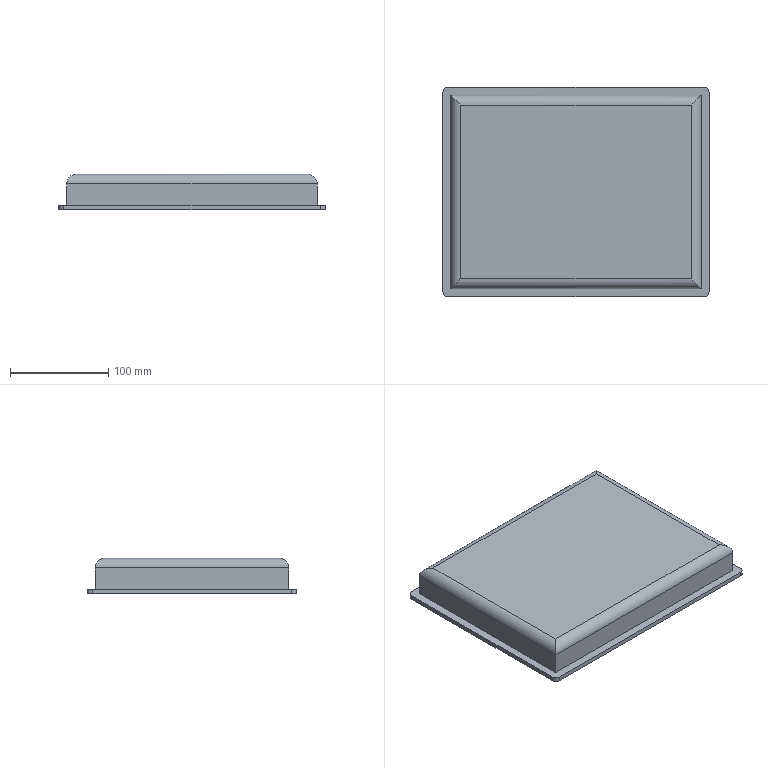Part | SolidWorks | features Fillet 2, ICE 2, Extrusion 1 | 1 solid | 24 faces | box 271 x 213 x 36.36 mm | volume 1748728 mm3 | plane 16 | cylinder 8 | commonest cylinder face diameters 10 x4 20 x4
STEP:
#1=CARTESIAN_POINT('',(0.,-5.,4.5));
#2=VERTEX_POINT('',#1);
#3=CARTESIAN_POINT('',(0.,-208.,4.5));
#4=VERTEX_POINT('',#3);
#5=CARTESIAN_POINT('',(0.,0.,4.5));
#6=DIRECTION('',(0.,-1.,0.));
#7=VECTOR('',#6,1000.);
#8=LINE('',#5,#7);
#9=EDGE_CURVE('',#2,#4,#8,.T.);
#10=ORIENTED_EDGE('',*,*,#9,.T.);
#11=CARTESIAN_POINT('',(5.,-213.,4.5));
#12=VERTEX_POINT('',#11);
#13=CARTESIAN_POINT('',(5.,-208.,4.5));
#14=DIRECTION('',(0.,0.,1.));
#15=DIRECTION('',(1.,0.,0.));
#16=AXIS2_PLACEMENT_3D('',#13,#14,#15);
#17=CIRCLE('',#16,5.);
#18=EDGE_CURVE('',#4,#12,#17,.T.);
#19=ORIENTED_EDGE('',*,*,#18,.T.);
#20=CARTESIAN_POINT('',(266.,-213.,4.5));
#21=VERTEX_POINT('',#20);
#22=CARTESIAN_POINT('',(0.,-213.,4.5));
#23=DIRECTION('',(1.,0.,0.));
#24=VECTOR('',#23,1000.);
#25=LINE('',#22,#24);
#26=EDGE_CURVE('',#12,#21,#25,.T.);
#27=ORIENTED_EDGE('',*,*,#26,.T.);
#28=CARTESIAN_POINT('',(271.,-208.,4.5));
#29=VERTEX_POINT('',#28);
#30=CARTESIAN_POINT('',(266.,-208.,4.5));
#31=DIRECTION('',(0.,0.,1.));
#32=DIRECTION('',(1.,0.,0.));
#33=AXIS2_PLACEMENT_3D('',#30,#31,#32);
#34=CIRCLE('',#33,5.);
#35=EDGE_CURVE('',#21,#29,#34,.T.);
#36=ORIENTED_EDGE('',*,*,#35,.T.);
#37=CARTESIAN_POINT('',(271.,-5.,4.5));
#38=VERTEX_POINT('',#37);
#39=CARTESIAN_POINT('',(271.,0.,4.5));
#40=DIRECTION('',(0.,1.,0.));
#41=VECTOR('',#40,1000.);
#42=LINE('',#39,#41);
#43=EDGE_CURVE('',#29,#38,#42,.T.);
#44=ORIENTED_EDGE('',*,*,#43,.T.);
#45=CARTESIAN_POINT('',(266.,0.,4.5));
#46=VERTEX_POINT('',#45);
#47=CARTESIAN_POINT('',(266.,-5.,4.5));
#48=DIRECTION('',(0.,0.,1.));
#49=DIRECTION('',(1.,0.,0.));
#50=AXIS2_PLACEMENT_3D('',#47,#48,#49);
#51=CIRCLE('',#50,5.);
#52=EDGE_CURVE('',#38,#46,#51,.T.);
#53=ORIENTED_EDGE('',*,*,#52,.T.);
#54=CARTESIAN_POINT('',(5.,0.,4.5));
#55=VERTEX_POINT('',#54);
#56=CARTESIAN_POINT('',(0.,0.,4.5));
#57=DIRECTION('',(-1.,0.,0.));
#58=VECTOR('',#57,1000.);
#59=LINE('',#56,#58);
#60=EDGE_CURVE('',#46,#55,#59,.T.);
#61=ORIENTED_EDGE('',*,*,#60,.T.);
#62=CARTESIAN_POINT('',(5.,-5.,4.5));
#63=DIRECTION('',(0.,0.,1.));
#64=DIRECTION('',(1.,0.,0.));
#65=AXIS2_PLACEMENT_3D('',#62,#63,#64);
#66=CIRCLE('',#65,5.);
#67=EDGE_CURVE('',#55,#2,#66,.T.);
#68=ORIENTED_EDGE('',*,*,#67,.T.);
#69=EDGE_LOOP('',(#10,#19,#27,#36,#44,#53,#61,#68));
#70=FACE_OUTER_BOUND('',#69,.T.);
#71=CARTESIAN_POINT('',(263.,-8.,4.5));
#72=VERTEX_POINT('',#71);
#73=CARTESIAN_POINT('',(8.,-8.,4.5));
#74=VERTEX_POINT('',#73);
#75=CARTESIAN_POINT('',(8.,-8.,4.5));
#76=DIRECTION('',(-1.,0.,0.));
#77=VECTOR('',#76,1000.);
#78=LINE('',#75,#77);
#79=EDGE_CURVE('',#72,#74,#78,.T.);
#80=ORIENTED_EDGE('',*,*,#79,.F.);
#81=CARTESIAN_POINT('',(263.,-205.,4.5));
#82=VERTEX_POINT('',#81);
#83=CARTESIAN_POINT('',(263.,-8.,4.5));
#84=DIRECTION('',(0.,1.,0.));
#85=VECTOR('',#84,1000.);
#86=LINE('',#83,#85);
#87=EDGE_CURVE('',#82,#72,#86,.T.);
#88=ORIENTED_EDGE('',*,*,#87,.F.);
#89=CARTESIAN_POINT('',(8.,-205.,4.5));
#90=VERTEX_POINT('',#89);
#91=CARTESIAN_POINT('',(8.,-205.,4.5));
#92=DIRECTION('',(1.,0.,0.));
#93=VECTOR('',#92,1000.);
#94=LINE('',#91,#93);
#95=EDGE_CURVE('',#90,#82,#94,.T.);
#96=ORIENTED_EDGE('',*,*,#95,.F.);
#97=CARTESIAN_POINT('',(8.,-8.,4.5));
#98=DIRECTION('',(0.,-1.,0.));
#99=VECTOR('',#98,1000.);
#100=LINE('',#97,#99);
#101=EDGE_CURVE('',#74,#90,#100,.T.);
#102=ORIENTED_EDGE('',*,*,#101,.F.);
#103=EDGE_LOOP('',(#80,#88,#96,#102));
#104=FACE_BOUND('',#103,.T.);
#105=CARTESIAN_POINT('',(0.,0.,4.5));
#106=DIRECTION('',(0.,0.,1.));
#107=DIRECTION('',(1.,0.,0.));
#108=AXIS2_PLACEMENT_3D('',#105,#106,#107);
#109=PLANE('',#108);
#110=ADVANCED_FACE('',(#70,#104),#109,.T.);
#111=CARTESIAN_POINT('',(0.,-5.,0.));
#112=VERTEX_POINT('',#111);
#113=CARTESIAN_POINT('',(0.,-208.,0.));
#114=VERTEX_POINT('',#113);
#115=CARTESIAN_POINT('',(0.,0.,0.));
#116=DIRECTION('',(0.,-1.,0.));
#117=VECTOR('',#116,1000.);
#118=LINE('',#115,#117);
#119=EDGE_CURVE('',#112,#114,#118,.T.);
#120=ORIENTED_EDGE('',*,*,#119,.T.);
#121=CARTESIAN_POINT('',(0.,-208.,4.5));
#122=DIRECTION('',(0.,0.,1.));
#123=VECTOR('',#122,1000.);
#124=LINE('',#121,#123);
#125=EDGE_CURVE('',#114,#4,#124,.T.);
#126=ORIENTED_EDGE('',*,*,#125,.T.);
#127=ORIENTED_EDGE('',*,*,#9,.F.);
#128=CARTESIAN_POINT('',(0.,-5.,4.5));
#129=DIRECTION('',(0.,0.,-1.));
#130=VECTOR('',#129,1000.);
#131=LINE('',#128,#130);
#132=EDGE_CURVE('',#2,#112,#131,.T.);
#133=ORIENTED_EDGE('',*,*,#132,.T.);
#134=EDGE_LOOP('',(#120,#126,#127,#133));
#135=FACE_OUTER_BOUND('',#134,.T.);
#136=CARTESIAN_POINT('',(0.,0.,4.5));
#137=DIRECTION('',(1.,0.,0.));
#138=DIRECTION('',(0.,1.,0.));
#139=AXIS2_PLACEMENT_3D('',#136,#137,#138);
#140=PLANE('',#139);
#141=ADVANCED_FACE('',(#135),#140,.F.);
#142=ORIENTED_EDGE('',*,*,#26,.F.);
#143=CARTESIAN_POINT('',(5.,-213.,0.));
#144=VERTEX_POINT('',#143);
#145=CARTESIAN_POINT('',(5.,-213.,4.5));
#146=DIRECTION('',(0.,0.,-1.));
#147=VECTOR('',#146,1000.);
#148=LINE('',#145,#147);
#149=EDGE_CURVE('',#12,#144,#148,.T.);
#150=ORIENTED_EDGE('',*,*,#149,.T.);
#151=CARTESIAN_POINT('',(266.,-213.,0.));
#152=VERTEX_POINT('',#151);
#153=CARTESIAN_POINT('',(0.,-213.,0.));
#154=DIRECTION('',(1.,0.,0.));
#155=VECTOR('',#154,1000.);
#156=LINE('',#153,#155);
#157=EDGE_CURVE('',#144,#152,#156,.T.);
#158=ORIENTED_EDGE('',*,*,#157,.T.);
#159=CARTESIAN_POINT('',(266.,-213.,4.5));
#160=DIRECTION('',(0.,0.,1.));
#161=VECTOR('',#160,1000.);
#162=LINE('',#159,#161);
#163=EDGE_CURVE('',#152,#21,#162,.T.);
#164=ORIENTED_EDGE('',*,*,#163,.T.);
#165=EDGE_LOOP('',(#142,#150,#158,#164));
#166=FACE_OUTER_BOUND('',#165,.T.);
#167=CARTESIAN_POINT('',(0.,-213.,4.5));
#168=DIRECTION('',(0.,1.,0.));
#169=DIRECTION('',(0.,0.,1.));
#170=AXIS2_PLACEMENT_3D('',#167,#168,#169);
#171=PLANE('',#170);
#172=ADVANCED_FACE('',(#166),#171,.F.);
#173=ORIENTED_EDGE('',*,*,#43,.F.);
#174=CARTESIAN_POINT('',(271.,-208.,0.));
#175=VERTEX_POINT('',#174);
#176=CARTESIAN_POINT('',(271.,-208.,4.5));
#177=DIRECTION('',(0.,0.,-1.));
#178=VECTOR('',#177,1000.);
#179=LINE('',#176,#178);
#180=EDGE_CURVE('',#29,#175,#179,.T.);
#181=ORIENTED_EDGE('',*,*,#180,.T.);
#182=CARTESIAN_POINT('',(271.,-5.,0.));
#183=VERTEX_POINT('',#182);
#184=CARTESIAN_POINT('',(271.,0.,0.));
#185=DIRECTION('',(0.,1.,0.));
#186=VECTOR('',#185,1000.);
#187=LINE('',#184,#186);
#188=EDGE_CURVE('',#175,#183,#187,.T.);
#189=ORIENTED_EDGE('',*,*,#188,.T.);
#190=CARTESIAN_POINT('',(271.,-5.,4.5));
#191=DIRECTION('',(0.,0.,1.));
#192=VECTOR('',#191,1000.);
#193=LINE('',#190,#192);
#194=EDGE_CURVE('',#183,#38,#193,.T.);
#195=ORIENTED_EDGE('',*,*,#194,.T.);
#196=EDGE_LOOP('',(#173,#181,#189,#195));
#197=FACE_OUTER_BOUND('',#196,.T.);
#198=CARTESIAN_POINT('',(271.,0.,4.5));
#199=DIRECTION('',(-1.,0.,0.));
#200=DIRECTION('',(0.,0.,1.));
#201=AXIS2_PLACEMENT_3D('',#198,#199,#200);
#202=PLANE('',#201);
#203=ADVANCED_FACE('',(#197),#202,.F.);
#204=ORIENTED_EDGE('',*,*,#60,.F.);
#205=CARTESIAN_POINT('',(266.,0.,0.));
#206=VERTEX_POINT('',#205);
#207=CARTESIAN_POINT('',(266.,0.,4.5));
#208=DIRECTION('',(0.,0.,-1.));
#209=VECTOR('',#208,1000.);
#210=LINE('',#207,#209);
#211=EDGE_CURVE('',#46,#206,#210,.T.);
#212=ORIENTED_EDGE('',*,*,#211,.T.);
#213=CARTESIAN_POINT('',(5.,0.,0.));
#214=VERTEX_POINT('',#213);
#215=CARTESIAN_POINT('',(0.,0.,0.));
#216=DIRECTION('',(-1.,0.,0.));
#217=VECTOR('',#216,1000.);
#218=LINE('',#215,#217);
#219=EDGE_CURVE('',#206,#214,#218,.T.);
#220=ORIENTED_EDGE('',*,*,#219,.T.);
#221=CARTESIAN_POINT('',(5.,0.,4.5));
#222=DIRECTION('',(0.,0.,1.));
#223=VECTOR('',#222,1000.);
#224=LINE('',#221,#223);
#225=EDGE_CURVE('',#214,#55,#224,.T.);
#226=ORIENTED_EDGE('',*,*,#225,.T.);
#227=EDGE_LOOP('',(#204,#212,#220,#226));
#228=FACE_OUTER_BOUND('',#227,.T.);
#229=CARTESIAN_POINT('',(0.,0.,4.5));
#230=DIRECTION('',(0.,-1.,0.));
#231=DIRECTION('',(0.,0.,-1.));
#232=AXIS2_PLACEMENT_3D('',#229,#230,#231);
#233=PLANE('',#232);
#234=ADVANCED_FACE('',(#228),#233,.F.);
#235=CARTESIAN_POINT('',(25.5,-36.5,0.));
#236=VERTEX_POINT('',#235);
#237=CARTESIAN_POINT('',(245.5,-36.5,0.));
#238=VERTEX_POINT('',#237);
#239=CARTESIAN_POINT('',(245.5,-36.5,0.));
#240=DIRECTION('',(1.,0.,0.));
#241=VECTOR('',#240,1000.);
#242=LINE('',#239,#241);
#243=EDGE_CURVE('',#236,#238,#242,.T.);
#244=ORIENTED_EDGE('',*,*,#243,.F.);
#245=CARTESIAN_POINT('',(25.5,-176.5,0.));
#246=VERTEX_POINT('',#245);
#247=CARTESIAN_POINT('',(25.5,-36.5,0.));
#248=DIRECTION('',(0.,1.,0.));
#249=VECTOR('',#248,1000.);
#250=LINE('',#247,#249);
#251=EDGE_CURVE('',#246,#236,#250,.T.);
#252=ORIENTED_EDGE('',*,*,#251,.F.);
#253=CARTESIAN_POINT('',(245.5,-176.5,0.));
#254=VERTEX_POINT('',#253);
#255=CARTESIAN_POINT('',(245.5,-176.5,0.));
#256=DIRECTION('',(-1.,0.,0.));
#257=VECTOR('',#256,1000.);
#258=LINE('',#255,#257);
#259=EDGE_CURVE('',#254,#246,#258,.T.);
#260=ORIENTED_EDGE('',*,*,#259,.F.);
#261=CARTESIAN_POINT('',(245.5,-36.5,0.));
#262=DIRECTION('',(0.,-1.,0.));
#263=VECTOR('',#262,1000.);
#264=LINE('',#261,#263);
#265=EDGE_CURVE('',#238,#254,#264,.T.);
#266=ORIENTED_EDGE('',*,*,#265,.F.);
#267=EDGE_LOOP('',(#244,#252,#260,#266));
#268=FACE_BOUND('',#267,.T.);
#269=ORIENTED_EDGE('',*,*,#157,.F.);
#270=CARTESIAN_POINT('',(5.,-208.,0.));
#271=DIRECTION('',(0.,0.,-1.));
#272=DIRECTION('',(1.,0.,0.));
#273=AXIS2_PLACEMENT_3D('',#270,#271,#272);
#274=CIRCLE('',#273,5.);
#275=EDGE_CURVE('',#144,#114,#274,.T.);
#276=ORIENTED_EDGE('',*,*,#275,.T.);
#277=ORIENTED_EDGE('',*,*,#119,.F.);
#278=CARTESIAN_POINT('',(5.,-5.,0.));
#279=DIRECTION('',(0.,0.,-1.));
#280=DIRECTION('',(1.,0.,0.));
#281=AXIS2_PLACEMENT_3D('',#278,#279,#280);
#282=CIRCLE('',#281,5.);
#283=EDGE_CURVE('',#112,#214,#282,.T.);
#284=ORIENTED_EDGE('',*,*,#283,.T.);
#285=ORIENTED_EDGE('',*,*,#219,.F.);
#286=CARTESIAN_POINT('',(266.,-5.,0.));
#287=DIRECTION('',(0.,0.,-1.));
#288=DIRECTION('',(1.,0.,0.));
#289=AXIS2_PLACEMENT_3D('',#286,#287,#288);
#290=CIRCLE('',#289,5.);
#291=EDGE_CURVE('',#206,#183,#290,.T.);
#292=ORIENTED_EDGE('',*,*,#291,.T.);
#293=ORIENTED_EDGE('',*,*,#188,.F.);
#294=CARTESIAN_POINT('',(266.,-208.,0.));
#295=DIRECTION('',(0.,0.,-1.));
#296=DIRECTION('',(1.,0.,0.));
#297=AXIS2_PLACEMENT_3D('',#294,#295,#296);
#298=CIRCLE('',#297,5.);
#299=EDGE_CURVE('',#175,#152,#298,.T.);
#300=ORIENTED_EDGE('',*,*,#299,.T.);
#301=EDGE_LOOP('',(#269,#276,#277,#284,#285,#292,#293,#300));
#302=FACE_OUTER_BOUND('',#301,.T.);
#303=CARTESIAN_POINT('',(0.,0.,0.));
#304=DIRECTION('',(0.,0.,1.));
#305=DIRECTION('',(1.,0.,0.));
#306=AXIS2_PLACEMENT_3D('',#303,#304,#305);
#307=PLANE('',#306);
#308=ADVANCED_FACE('',(#268,#302),#307,.F.);
#309=CARTESIAN_POINT('',(263.,-8.,26.36));
#310=VERTEX_POINT('',#309);
#311=CARTESIAN_POINT('',(263.,-8.,36.36));
#312=DIRECTION('',(0.,0.,-1.));
#313=VECTOR('',#312,1000.);
#314=LINE('',#311,#313);
#315=EDGE_CURVE('',#310,#72,#314,.T.);
#316=ORIENTED_EDGE('',*,*,#315,.F.);
#317=CARTESIAN_POINT('',(263.,-205.,26.36));
#318=VERTEX_POINT('',#317);
#319=CARTESIAN_POINT('',(263.,-205.,26.36));
#320=DIRECTION('',(0.,-1.,0.));
#321=VECTOR('',#320,1000.);
#322=LINE('',#319,#321);
#323=EDGE_CURVE('',#310,#318,#322,.T.);
#324=ORIENTED_EDGE('',*,*,#323,.T.);
#325=CARTESIAN_POINT('',(263.,-205.,36.36));
#326=DIRECTION('',(0.,0.,-1.));
#327=VECTOR('',#326,1000.);
#328=LINE('',#325,#327);
#329=EDGE_CURVE('',#318,#82,#328,.T.);
#330=ORIENTED_EDGE('',*,*,#329,.T.);
#331=ORIENTED_EDGE('',*,*,#87,.T.);
#332=EDGE_LOOP('',(#316,#324,#330,#331));
#333=FACE_OUTER_BOUND('',#332,.T.);
#334=CARTESIAN_POINT('',(263.,-8.,36.36));
#335=DIRECTION('',(-1.,0.,0.));
#336=DIRECTION('',(0.,0.,1.));
#337=AXIS2_PLACEMENT_3D('',#334,#335,#336);
#338=PLANE('',#337);
#339=ADVANCED_FACE('',(#333),#338,.F.);
#340=CARTESIAN_POINT('',(8.,-8.,26.36));
#341=VERTEX_POINT('',#340);
#342=CARTESIAN_POINT('',(8.,-8.,36.36));
#343=DIRECTION('',(0.,0.,-1.));
#344=VECTOR('',#343,1000.);
#345=LINE('',#342,#344);
#346=EDGE_CURVE('',#341,#74,#345,.T.);
#347=ORIENTED_EDGE('',*,*,#346,.F.);
#348=CARTESIAN_POINT('',(263.,-8.,26.36));
#349=DIRECTION('',(1.,0.,0.));
#350=VECTOR('',#349,1000.);
#351=LINE('',#348,#350);
#352=EDGE_CURVE('',#341,#310,#351,.T.);
#353=ORIENTED_EDGE('',*,*,#352,.T.);
#354=ORIENTED_EDGE('',*,*,#315,.T.);
#355=ORIENTED_EDGE('',*,*,#79,.T.);
#356=EDGE_LOOP('',(#347,#353,#354,#355));
#357=FACE_OUTER_BOUND('',#356,.T.);
#358=CARTESIAN_POINT('',(8.,-8.,36.36));
#359=DIRECTION('',(0.,-1.,0.));
#360=DIRECTION('',(0.,0.,-1.));
#361=AXIS2_PLACEMENT_3D('',#358,#359,#360);
#362=PLANE('',#361);
#363=ADVANCED_FACE('',(#357),#362,.F.);
#364=CARTESIAN_POINT('',(8.,-205.,26.36));
#365=VERTEX_POINT('',#364);
#366=CARTESIAN_POINT('',(8.,-205.,36.36));
#367=DIRECTION('',(0.,0.,-1.));
#368=VECTOR('',#367,1000.);
#369=LINE('',#366,#368);
#370=EDGE_CURVE('',#365,#90,#369,.T.);
#371=ORIENTED_EDGE('',*,*,#370,.F.);
#372=CARTESIAN_POINT('',(8.,-8.,26.36));
#373=DIRECTION('',(0.,1.,0.));
#374=VECTOR('',#373,1000.);
#375=LINE('',#372,#374);
#376=EDGE_CURVE('',#365,#341,#375,.T.);
#377=ORIENTED_EDGE('',*,*,#376,.T.);
#378=ORIENTED_EDGE('',*,*,#346,.T.);
#379=ORIENTED_EDGE('',*,*,#101,.T.);
#380=EDGE_LOOP('',(#371,#377,#378,#379));
#381=FACE_OUTER_BOUND('',#380,.T.);
#382=CARTESIAN_POINT('',(8.,-8.,36.36));
#383=DIRECTION('',(1.,0.,0.));
#384=DIRECTION('',(0.,1.,0.));
#385=AXIS2_PLACEMENT_3D('',#382,#383,#384);
#386=PLANE('',#385);
#387=ADVANCED_FACE('',(#381),#386,.F.);
#388=ORIENTED_EDGE('',*,*,#329,.F.);
#389=CARTESIAN_POINT('',(8.,-205.,26.36));
#390=DIRECTION('',(-1.,0.,0.));
#391=VECTOR('',#390,1000.);
#392=LINE('',#389,#391);
#393=EDGE_CURVE('',#318,#365,#392,.T.);
#394=ORIENTED_EDGE('',*,*,#393,.T.);
#395=ORIENTED_EDGE('',*,*,#370,.T.);
#396=ORIENTED_EDGE('',*,*,#95,.T.);
#397=EDGE_LOOP('',(#388,#394,#395,#396));
#398=FACE_OUTER_BOUND('',#397,.T.);
#399=CARTESIAN_POINT('',(8.,-205.,36.36));
#400=DIRECTION('',(0.,1.,0.));
#401=DIRECTION('',(0.,0.,1.));
#402=AXIS2_PLACEMENT_3D('',#399,#400,#401);
#403=PLANE('',#402);
#404=ADVANCED_FACE('',(#398),#403,.F.);
#405=CARTESIAN_POINT('',(18.,-18.,36.36));
#406=VERTEX_POINT('',#405);
#407=CARTESIAN_POINT('',(18.,-195.,36.36));
#408=VERTEX_POINT('',#407);
#409=CARTESIAN_POINT('',(18.,-205.,36.36));
#410=DIRECTION('',(0.,-1.,0.));
#411=VECTOR('',#410,1000.);
#412=LINE('',#409,#411);
#413=EDGE_CURVE('',#406,#408,#412,.T.);
#414=ORIENTED_EDGE('',*,*,#413,.T.);
#415=CARTESIAN_POINT('',(253.,-195.,36.36));
#416=VERTEX_POINT('',#415);
#417=CARTESIAN_POINT('',(263.,-195.,36.36));
#418=DIRECTION('',(1.,0.,0.));
#419=VECTOR('',#418,1000.);
#420=LINE('',#417,#419);
#421=EDGE_CURVE('',#408,#416,#420,.T.);
#422=ORIENTED_EDGE('',*,*,#421,.T.);
#423=CARTESIAN_POINT('',(253.,-18.,36.36));
#424=VERTEX_POINT('',#423);
#425=CARTESIAN_POINT('',(253.,-8.,36.36));
#426=DIRECTION('',(0.,1.,0.));
#427=VECTOR('',#426,1000.);
#428=LINE('',#425,#427);
#429=EDGE_CURVE('',#416,#424,#428,.T.);
#430=ORIENTED_EDGE('',*,*,#429,.T.);
#431=CARTESIAN_POINT('',(8.,-18.,36.36));
#432=DIRECTION('',(-1.,0.,0.));
#433=VECTOR('',#432,1000.);
#434=LINE('',#431,#433);
#435=EDGE_CURVE('',#424,#406,#434,.T.);
#436=ORIENTED_EDGE('',*,*,#435,.T.);
#437=EDGE_LOOP('',(#414,#422,#430,#436));
#438=FACE_OUTER_BOUND('',#437,.T.);
#439=CARTESIAN_POINT('',(0.,0.,36.36));
#440=DIRECTION('',(0.,0.,1.));
#441=DIRECTION('',(1.,0.,0.));
#442=AXIS2_PLACEMENT_3D('',#439,#440,#441);
#443=PLANE('',#442);
#444=ADVANCED_FACE('',(#438),#443,.T.);
#445=CARTESIAN_POINT('',(263.,-8.,26.36));
#446=CARTESIAN_POINT('',(263.,-8.,32.218));
#447=CARTESIAN_POINT('',(258.858,-12.142,36.36));
#448=CARTESIAN_POINT('',(253.,-18.,36.36));
#449=(BOUNDED_CURVE()B_SPLINE_CURVE(3,(#445,#446,#447,#448),.UNSPECIFIED.,.F.,.F.)B_SPLINE_CURVE_WITH_KNOTS((4,4),(3.142,4.712),.UNSPECIFIED.)CURVE()GEOMETRIC_REPRESENTATION_ITEM()RATIONAL_B_SPLINE_CURVE((1.,0.8047,0.8047,1.))REPRESENTATION_ITEM(''));
#450=EDGE_CURVE('',#310,#424,#449,.T.);
#451=ORIENTED_EDGE('',*,*,#450,.F.);
#452=ORIENTED_EDGE('',*,*,#352,.F.);
#453=CARTESIAN_POINT('',(18.,-18.,36.36));
#454=CARTESIAN_POINT('',(12.142,-12.142,36.36));
#455=CARTESIAN_POINT('',(8.,-8.,32.218));
#456=CARTESIAN_POINT('',(8.,-8.,26.36));
#457=(BOUNDED_CURVE()B_SPLINE_CURVE(3,(#453,#454,#455,#456),.UNSPECIFIED.,.F.,.F.)B_SPLINE_CURVE_WITH_KNOTS((4,4),(1.571,3.142),.UNSPECIFIED.)CURVE()GEOMETRIC_REPRESENTATION_ITEM()RATIONAL_B_SPLINE_CURVE((1.,0.8047,0.8047,1.))REPRESENTATION_ITEM(''));
#458=EDGE_CURVE('',#406,#341,#457,.T.);
#459=ORIENTED_EDGE('',*,*,#458,.F.);
#460=ORIENTED_EDGE('',*,*,#435,.F.);
#461=EDGE_LOOP('',(#451,#452,#459,#460));
#462=FACE_OUTER_BOUND('',#461,.T.);
#463=CARTESIAN_POINT('',(0.,-18.,26.36));
#464=DIRECTION('',(1.,0.,0.));
#465=DIRECTION('',(0.,0.,-1.));
#466=AXIS2_PLACEMENT_3D('',#463,#464,#465);
#467=CYLINDRICAL_SURFACE('',#466,10.);
#468=ADVANCED_FACE('',(#462),#467,.T.);
#469=ORIENTED_EDGE('',*,*,#458,.T.);
#470=ORIENTED_EDGE('',*,*,#376,.F.);
#471=CARTESIAN_POINT('',(18.,-195.,36.36));
#472=CARTESIAN_POINT('',(12.142,-200.858,36.36));
#473=CARTESIAN_POINT('',(8.,-205.,32.218));
#474=CARTESIAN_POINT('',(8.,-205.,26.36));
#475=(BOUNDED_CURVE()B_SPLINE_CURVE(3,(#471,#472,#473,#474),.UNSPECIFIED.,.F.,.F.)B_SPLINE_CURVE_WITH_KNOTS((4,4),(1.571,3.142),.UNSPECIFIED.)CURVE()GEOMETRIC_REPRESENTATION_ITEM()RATIONAL_B_SPLINE_CURVE((1.,0.8047,0.8047,1.))REPRESENTATION_ITEM(''));
#476=EDGE_CURVE('',#408,#365,#475,.T.);
#477=ORIENTED_EDGE('',*,*,#476,.F.);
#478=ORIENTED_EDGE('',*,*,#413,.F.);
#479=EDGE_LOOP('',(#469,#470,#477,#478));
#480=FACE_OUTER_BOUND('',#479,.T.);
#481=CARTESIAN_POINT('',(18.,0.,26.36));
#482=DIRECTION('',(0.,1.,0.));
#483=DIRECTION('',(-1.,0.,0.));
#484=AXIS2_PLACEMENT_3D('',#481,#482,#483);
#485=CYLINDRICAL_SURFACE('',#484,10.);
#486=ADVANCED_FACE('',(#480),#485,.T.);
#487=ORIENTED_EDGE('',*,*,#450,.T.);
#488=ORIENTED_EDGE('',*,*,#429,.F.);
#489=CARTESIAN_POINT('',(263.,-205.,26.36));
#490=CARTESIAN_POINT('',(263.,-205.,32.218));
#491=CARTESIAN_POINT('',(258.858,-200.858,36.36));
#492=CARTESIAN_POINT('',(253.,-195.,36.36));
#493=(BOUNDED_CURVE()B_SPLINE_CURVE(3,(#489,#490,#491,#492),.UNSPECIFIED.,.F.,.F.)B_SPLINE_CURVE_WITH_KNOTS((4,4),(0.,1.571),.UNSPECIFIED.)CURVE()GEOMETRIC_REPRESENTATION_ITEM()RATIONAL_B_SPLINE_CURVE((1.,0.8047,0.8047,1.))REPRESENTATION_ITEM(''));
#494=EDGE_CURVE('',#318,#416,#493,.T.);
#495=ORIENTED_EDGE('',*,*,#494,.F.);
#496=ORIENTED_EDGE('',*,*,#323,.F.);
#497=EDGE_LOOP('',(#487,#488,#495,#496));
#498=FACE_OUTER_BOUND('',#497,.T.);
#499=CARTESIAN_POINT('',(253.,0.,26.36));
#500=DIRECTION('',(0.,-1.,0.));
#501=DIRECTION('',(0.,0.,-1.));
#502=AXIS2_PLACEMENT_3D('',#499,#500,#501);
#503=CYLINDRICAL_SURFACE('',#502,10.);
#504=ADVANCED_FACE('',(#498),#503,.T.);
#505=ORIENTED_EDGE('',*,*,#476,.T.);
#506=ORIENTED_EDGE('',*,*,#393,.F.);
#507=ORIENTED_EDGE('',*,*,#494,.T.);
#508=ORIENTED_EDGE('',*,*,#421,.F.);
#509=EDGE_LOOP('',(#505,#506,#507,#508));
#510=FACE_OUTER_BOUND('',#509,.T.);
#511=CARTESIAN_POINT('',(0.,-195.,26.36));
#512=DIRECTION('',(-1.,0.,0.));
#513=DIRECTION('',(0.,0.,1.));
#514=AXIS2_PLACEMENT_3D('',#511,#512,#513);
#515=CYLINDRICAL_SURFACE('',#514,10.);
#516=ADVANCED_FACE('',(#510),#515,.T.);
#517=ORIENTED_EDGE('',*,*,#18,.F.);
#518=ORIENTED_EDGE('',*,*,#125,.F.);
#519=ORIENTED_EDGE('',*,*,#275,.F.);
#520=ORIENTED_EDGE('',*,*,#149,.F.);
#521=EDGE_LOOP('',(#517,#518,#519,#520));
#522=FACE_OUTER_BOUND('',#521,.T.);
#523=CARTESIAN_POINT('',(5.,-208.,4.5));
#524=DIRECTION('',(0.,0.,-1.));
#525=DIRECTION('',(-1.,0.,0.));
#526=AXIS2_PLACEMENT_3D('',#523,#524,#525);
#527=CYLINDRICAL_SURFACE('',#526,5.);
#528=ADVANCED_FACE('',(#522),#527,.T.);
#529=ORIENTED_EDGE('',*,*,#35,.F.);
#530=ORIENTED_EDGE('',*,*,#163,.F.);
#531=ORIENTED_EDGE('',*,*,#299,.F.);
#532=ORIENTED_EDGE('',*,*,#180,.F.);
#533=EDGE_LOOP('',(#529,#530,#531,#532));
#534=FACE_OUTER_BOUND('',#533,.T.);
#535=CARTESIAN_POINT('',(266.,-208.,4.5));
#536=DIRECTION('',(0.,0.,-1.));
#537=DIRECTION('',(-1.,0.,0.));
#538=AXIS2_PLACEMENT_3D('',#535,#536,#537);
#539=CYLINDRICAL_SURFACE('',#538,5.);
#540=ADVANCED_FACE('',(#534),#539,.T.);
#541=ORIENTED_EDGE('',*,*,#52,.F.);
#542=ORIENTED_EDGE('',*,*,#194,.F.);
#543=ORIENTED_EDGE('',*,*,#291,.F.);
#544=ORIENTED_EDGE('',*,*,#211,.F.);
#545=EDGE_LOOP('',(#541,#542,#543,#544));
#546=FACE_OUTER_BOUND('',#545,.T.);
#547=CARTESIAN_POINT('',(266.,-5.,4.5));
#548=DIRECTION('',(0.,0.,-1.));
#549=DIRECTION('',(-1.,0.,0.));
#550=AXIS2_PLACEMENT_3D('',#547,#548,#549);
#551=CYLINDRICAL_SURFACE('',#550,5.);
#552=ADVANCED_FACE('',(#546),#551,.T.);
#553=ORIENTED_EDGE('',*,*,#67,.F.);
#554=ORIENTED_EDGE('',*,*,#225,.F.);
#555=ORIENTED_EDGE('',*,*,#283,.F.);
#556=ORIENTED_EDGE('',*,*,#132,.F.);
#557=EDGE_LOOP('',(#553,#554,#555,#556));
#558=FACE_OUTER_BOUND('',#557,.T.);
#559=CARTESIAN_POINT('',(5.,-5.,4.5));
#560=DIRECTION('',(0.,0.,-1.));
#561=DIRECTION('',(-1.,0.,0.));
#562=AXIS2_PLACEMENT_3D('',#559,#560,#561);
#563=CYLINDRICAL_SURFACE('',#562,5.);
#564=ADVANCED_FACE('',(#558),#563,.T.);
#565=ORIENTED_EDGE('',*,*,#251,.T.);
#566=CARTESIAN_POINT('',(25.5,-36.5,3.));
#567=VERTEX_POINT('',#566);
#568=CARTESIAN_POINT('',(25.5,-36.5,3.));
#569=DIRECTION('',(0.,0.,-1.));
#570=VECTOR('',#569,1000.);
#571=LINE('',#568,#570);
#572=EDGE_CURVE('',#567,#236,#571,.T.);
#573=ORIENTED_EDGE('',*,*,#572,.F.);
#574=CARTESIAN_POINT('',(25.5,-176.5,3.));
#575=VERTEX_POINT('',#574);
#576=CARTESIAN_POINT('',(25.5,-36.5,3.));
#577=DIRECTION('',(0.,1.,0.));
#578=VECTOR('',#577,1000.);
#579=LINE('',#576,#578);
#580=EDGE_CURVE('',#575,#567,#579,.T.);
#581=ORIENTED_EDGE('',*,*,#580,.F.);
#582=CARTESIAN_POINT('',(25.5,-176.5,3.));
#583=DIRECTION('',(0.,0.,-1.));
#584=VECTOR('',#583,1000.);
#585=LINE('',#582,#584);
#586=EDGE_CURVE('',#575,#246,#585,.T.);
#587=ORIENTED_EDGE('',*,*,#586,.T.);
#588=EDGE_LOOP('',(#565,#573,#581,#587));
#589=FACE_OUTER_BOUND('',#588,.T.);
#590=CARTESIAN_POINT('',(25.5,-36.5,3.));
#591=DIRECTION('',(-1.,0.,0.));
#592=DIRECTION('',(0.,-1.,0.));
#593=AXIS2_PLACEMENT_3D('',#590,#591,#592);
#594=PLANE('',#593);
#595=ADVANCED_FACE('',(#589),#594,.F.);
#596=ORIENTED_EDGE('',*,*,#259,.T.);
#597=ORIENTED_EDGE('',*,*,#586,.F.);
#598=CARTESIAN_POINT('',(245.5,-176.5,3.));
#599=VERTEX_POINT('',#598);
#600=CARTESIAN_POINT('',(245.5,-176.5,3.));
#601=DIRECTION('',(-1.,0.,0.));
#602=VECTOR('',#601,1000.);
#603=LINE('',#600,#602);
#604=EDGE_CURVE('',#599,#575,#603,.T.);
#605=ORIENTED_EDGE('',*,*,#604,.F.);
#606=CARTESIAN_POINT('',(245.5,-176.5,3.));
#607=DIRECTION('',(0.,0.,-1.));
#608=VECTOR('',#607,1000.);
#609=LINE('',#606,#608);
#610=EDGE_CURVE('',#599,#254,#609,.T.);
#611=ORIENTED_EDGE('',*,*,#610,.T.);
#612=EDGE_LOOP('',(#596,#597,#605,#611));
#613=FACE_OUTER_BOUND('',#612,.T.);
#614=CARTESIAN_POINT('',(245.5,-176.5,3.));
#615=DIRECTION('',(0.,-1.,0.));
#616=DIRECTION('',(0.,0.,-1.));
#617=AXIS2_PLACEMENT_3D('',#614,#615,#616);
#618=PLANE('',#617);
#619=ADVANCED_FACE('',(#613),#618,.F.);
#620=ORIENTED_EDGE('',*,*,#265,.T.);
#621=ORIENTED_EDGE('',*,*,#610,.F.);
#622=CARTESIAN_POINT('',(245.5,-36.5,3.));
#623=VERTEX_POINT('',#622);
#624=CARTESIAN_POINT('',(245.5,-36.5,3.));
#625=DIRECTION('',(0.,-1.,0.));
#626=VECTOR('',#625,1000.);
#627=LINE('',#624,#626);
#628=EDGE_CURVE('',#623,#599,#627,.T.);
#629=ORIENTED_EDGE('',*,*,#628,.F.);
#630=CARTESIAN_POINT('',(245.5,-36.5,3.));
#631=DIRECTION('',(0.,0.,-1.));
#632=VECTOR('',#631,1000.);
#633=LINE('',#630,#632);
#634=EDGE_CURVE('',#623,#238,#633,.T.);
#635=ORIENTED_EDGE('',*,*,#634,.T.);
#636=EDGE_LOOP('',(#620,#621,#629,#635));
#637=FACE_OUTER_BOUND('',#636,.T.);
#638=CARTESIAN_POINT('',(245.5,-36.5,3.));
#639=DIRECTION('',(1.,0.,0.));
#640=DIRECTION('',(0.,1.,0.));
#641=AXIS2_PLACEMENT_3D('',#638,#639,#640);
#642=PLANE('',#641);
#643=ADVANCED_FACE('',(#637),#642,.F.);
#644=ORIENTED_EDGE('',*,*,#243,.T.);
#645=ORIENTED_EDGE('',*,*,#634,.F.);
#646=CARTESIAN_POINT('',(245.5,-36.5,3.));
#647=DIRECTION('',(1.,0.,0.));
#648=VECTOR('',#647,1000.);
#649=LINE('',#646,#648);
#650=EDGE_CURVE('',#567,#623,#649,.T.);
#651=ORIENTED_EDGE('',*,*,#650,.F.);
#652=ORIENTED_EDGE('',*,*,#572,.T.);
#653=EDGE_LOOP('',(#644,#645,#651,#652));
#654=FACE_OUTER_BOUND('',#653,.T.);
#655=CARTESIAN_POINT('',(245.5,-36.5,3.));
#656=DIRECTION('',(0.,1.,0.));
#657=DIRECTION('',(0.,0.,1.));
#658=AXIS2_PLACEMENT_3D('',#655,#656,#657);
#659=PLANE('',#658);
#660=ADVANCED_FACE('',(#654),#659,.F.);
#661=ORIENTED_EDGE('',*,*,#580,.T.);
#662=ORIENTED_EDGE('',*,*,#650,.T.);
#663=ORIENTED_EDGE('',*,*,#628,.T.);
#664=ORIENTED_EDGE('',*,*,#604,.T.);
#665=EDGE_LOOP('',(#661,#662,#663,#664));
#666=FACE_OUTER_BOUND('',#665,.T.);
#667=CARTESIAN_POINT('',(0.,0.,3.));
#668=DIRECTION('',(0.,0.,-1.));
#669=DIRECTION('',(-1.,0.,0.));
#670=AXIS2_PLACEMENT_3D('',#667,#668,#669);
#671=PLANE('',#670);
#672=ADVANCED_FACE('',(#666),#671,.T.);
#673=CLOSED_SHELL('',(#110,#141,#172,#203,#234,#308,#339,#363,#387,#404,#444,#468,#486,#504,#516,#528,#540,#552,#564,#595,#619,#643,#660,#672));
#674=MANIFOLD_SOLID_BREP('',#673);
#675=CARTESIAN_POINT('',(0.,0.,0.));
#676=DIRECTION('',(0.,0.,1.));
#677=DIRECTION('',(1.,0.,0.));
#678=AXIS2_PLACEMENT_3D('',#675,#676,#677);
#679=(LENGTH_UNIT()NAMED_UNIT(*)SI_UNIT(.MILLI.,.METRE.));
#680=UNCERTAINTY_MEASURE_WITH_UNIT(LENGTH_MEASURE(0.00001),#679,'','');
#681=(NAMED_UNIT(*)PLANE_ANGLE_UNIT()SI_UNIT($,.RADIAN.));
#682=(NAMED_UNIT(*)SI_UNIT($,.STERADIAN.)SOLID_ANGLE_UNIT());
#683=(GEOMETRIC_REPRESENTATION_CONTEXT(3)GLOBAL_UNCERTAINTY_ASSIGNED_CONTEXT((#680))GLOBAL_UNIT_ASSIGNED_CONTEXT((#679,#681,#682))REPRESENTATION_CONTEXT('',''));
#684=ADVANCED_BREP_SHAPE_REPRESENTATION('',(#674,#678),#683);